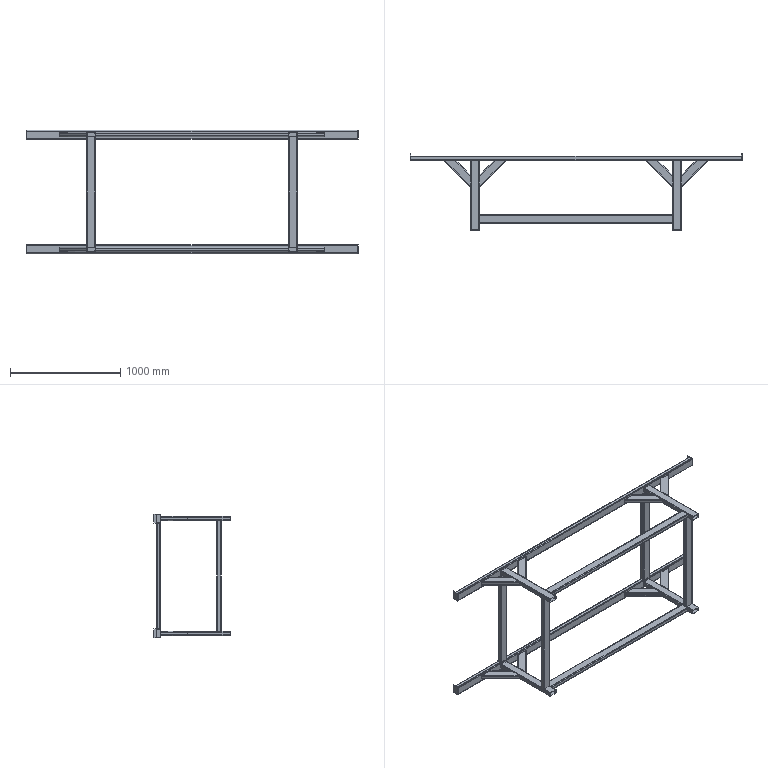Part | SolidWorks | features ICE 2, WeldCornerFeat 2, 3DProfileFeature 1, WeldMemberFeat 1, WeldmentFeature 1 | 24 solids | 384 faces | box 3010 x 690 x 1120 mm | volume 15558930 mm3 | plane 224 | cylinder 160 | commonest cylinder face diameters 8 x80 16 x80